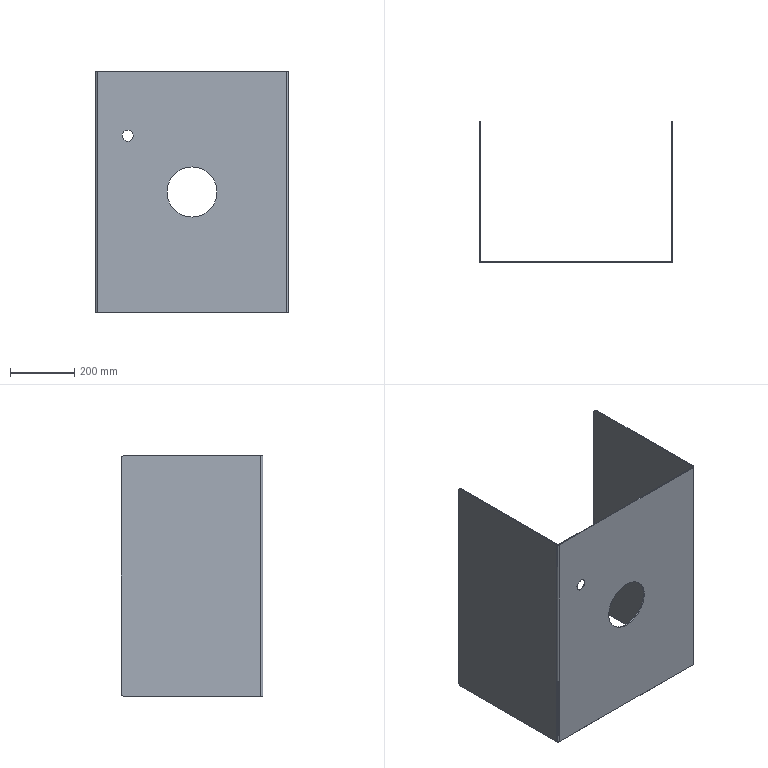Part | SolidWorks | features ICE 2, FlatPattern 1, SMBaseFlange 1, SheetMetal 1 | 1 solid | 30 faces | box 600 x 440 x 750 mm | volume 3247324 mm3 | plane 18 | cylinder 12 | commonest cylinder face diameters 20 x4 6 x2 12 x2 35 x2 156 x2
STEP:
#1=CARTESIAN_POINT('',(300.,0.,297.));
#2=VERTEX_POINT('',#1);
#3=CARTESIAN_POINT('',(300.,0.,453.));
#4=VERTEX_POINT('',#3);
#5=CARTESIAN_POINT('',(300.,0.,375.));
#6=DIRECTION('',(0.,1.,0.));
#7=DIRECTION('',(0.,0.,1.));
#8=AXIS2_PLACEMENT_3D('',#5,#6,#7);
#9=CIRCLE('',#8,78.);
#10=EDGE_CURVE('',#2,#4,#9,.T.);
#11=ORIENTED_EDGE('',*,*,#10,.F.);
#12=CARTESIAN_POINT('',(300.,3.,297.));
#13=VERTEX_POINT('',#12);
#14=CARTESIAN_POINT('',(300.,-7.,297.));
#15=DIRECTION('',(0.,1.,0.));
#16=VECTOR('',#15,1000.);
#17=LINE('',#14,#16);
#18=EDGE_CURVE('',#2,#13,#17,.T.);
#19=ORIENTED_EDGE('',*,*,#18,.T.);
#20=CARTESIAN_POINT('',(300.,3.,453.));
#21=VERTEX_POINT('',#20);
#22=CARTESIAN_POINT('',(300.,3.,375.));
#23=DIRECTION('',(0.,1.,0.));
#24=DIRECTION('',(0.,0.,1.));
#25=AXIS2_PLACEMENT_3D('',#22,#23,#24);
#26=CIRCLE('',#25,78.);
#27=EDGE_CURVE('',#13,#21,#26,.T.);
#28=ORIENTED_EDGE('',*,*,#27,.T.);
#29=CARTESIAN_POINT('',(300.,-7.,453.));
#30=DIRECTION('',(0.,1.,0.));
#31=VECTOR('',#30,1000.);
#32=LINE('',#29,#31);
#33=EDGE_CURVE('',#4,#21,#32,.T.);
#34=ORIENTED_EDGE('',*,*,#33,.F.);
#35=EDGE_LOOP('',(#11,#19,#28,#34));
#36=FACE_OUTER_BOUND('',#35,.T.);
#37=CARTESIAN_POINT('',(300.,-7.,375.));
#38=DIRECTION('',(0.,1.,0.));
#39=DIRECTION('',(0.,0.,1.));
#40=AXIS2_PLACEMENT_3D('',#37,#38,#39);
#41=CYLINDRICAL_SURFACE('',#40,78.);
#42=ADVANCED_FACE('',(#36),#41,.F.);
#43=CARTESIAN_POINT('',(100.,0.,532.5));
#44=VERTEX_POINT('',#43);
#45=CARTESIAN_POINT('',(100.,0.,567.5));
#46=VERTEX_POINT('',#45);
#47=CARTESIAN_POINT('',(100.,0.,550.));
#48=DIRECTION('',(0.,1.,0.));
#49=DIRECTION('',(0.,0.,1.));
#50=AXIS2_PLACEMENT_3D('',#47,#48,#49);
#51=CIRCLE('',#50,17.5);
#52=EDGE_CURVE('',#44,#46,#51,.T.);
#53=ORIENTED_EDGE('',*,*,#52,.F.);
#54=CARTESIAN_POINT('',(100.,3.,532.5));
#55=VERTEX_POINT('',#54);
#56=CARTESIAN_POINT('',(100.,-7.,532.5));
#57=DIRECTION('',(0.,1.,0.));
#58=VECTOR('',#57,1000.);
#59=LINE('',#56,#58);
#60=EDGE_CURVE('',#44,#55,#59,.T.);
#61=ORIENTED_EDGE('',*,*,#60,.T.);
#62=CARTESIAN_POINT('',(100.,3.,567.5));
#63=VERTEX_POINT('',#62);
#64=CARTESIAN_POINT('',(100.,3.,550.));
#65=DIRECTION('',(0.,1.,0.));
#66=DIRECTION('',(0.,0.,1.));
#67=AXIS2_PLACEMENT_3D('',#64,#65,#66);
#68=CIRCLE('',#67,17.5);
#69=EDGE_CURVE('',#55,#63,#68,.T.);
#70=ORIENTED_EDGE('',*,*,#69,.T.);
#71=CARTESIAN_POINT('',(100.,-7.,567.5));
#72=DIRECTION('',(0.,1.,0.));
#73=VECTOR('',#72,1000.);
#74=LINE('',#71,#73);
#75=EDGE_CURVE('',#46,#63,#74,.T.);
#76=ORIENTED_EDGE('',*,*,#75,.F.);
#77=EDGE_LOOP('',(#53,#61,#70,#76));
#78=FACE_OUTER_BOUND('',#77,.T.);
#79=CARTESIAN_POINT('',(100.,-7.,550.));
#80=DIRECTION('',(0.,1.,0.));
#81=DIRECTION('',(0.,0.,1.));
#82=AXIS2_PLACEMENT_3D('',#79,#80,#81);
#83=CYLINDRICAL_SURFACE('',#82,17.5);
#84=ADVANCED_FACE('',(#78),#83,.F.);
#85=CARTESIAN_POINT('',(600.,430.,0.));
#86=VERTEX_POINT('',#85);
#87=CARTESIAN_POINT('',(600.,440.,10.));
#88=VERTEX_POINT('',#87);
#89=CARTESIAN_POINT('',(600.,430.,10.));
#90=DIRECTION('',(1.,0.,0.));
#91=DIRECTION('',(0.,0.,1.));
#92=AXIS2_PLACEMENT_3D('',#89,#90,#91);
#93=CIRCLE('',#92,10.);
#94=EDGE_CURVE('',#86,#88,#93,.T.);
#95=ORIENTED_EDGE('',*,*,#94,.T.);
#96=CARTESIAN_POINT('',(600.,440.,740.));
#97=VERTEX_POINT('',#96);
#98=CARTESIAN_POINT('',(600.,440.,750.));
#99=DIRECTION('',(0.,0.,-1.));
#100=VECTOR('',#99,1000.);
#101=LINE('',#98,#100);
#102=EDGE_CURVE('',#97,#88,#101,.T.);
#103=ORIENTED_EDGE('',*,*,#102,.F.);
#104=CARTESIAN_POINT('',(600.,430.,750.));
#105=VERTEX_POINT('',#104);
#106=CARTESIAN_POINT('',(600.,430.,740.));
#107=DIRECTION('',(1.,0.,0.));
#108=DIRECTION('',(0.,0.,1.));
#109=AXIS2_PLACEMENT_3D('',#106,#107,#108);
#110=CIRCLE('',#109,10.);
#111=EDGE_CURVE('',#97,#105,#110,.T.);
#112=ORIENTED_EDGE('',*,*,#111,.T.);
#113=CARTESIAN_POINT('',(600.,6.,750.));
#114=VERTEX_POINT('',#113);
#115=CARTESIAN_POINT('',(600.,0.,750.));
#116=DIRECTION('',(0.,1.,0.));
#117=VECTOR('',#116,1000.);
#118=LINE('',#115,#117);
#119=EDGE_CURVE('',#114,#105,#118,.T.);
#120=ORIENTED_EDGE('',*,*,#119,.F.);
#121=CARTESIAN_POINT('',(600.,6.,0.));
#122=VERTEX_POINT('',#121);
#123=CARTESIAN_POINT('',(600.,6.,750.));
#124=DIRECTION('',(0.,0.,-1.));
#125=VECTOR('',#124,1000.);
#126=LINE('',#123,#125);
#127=EDGE_CURVE('',#114,#122,#126,.T.);
#128=ORIENTED_EDGE('',*,*,#127,.T.);
#129=CARTESIAN_POINT('',(600.,0.,0.));
#130=DIRECTION('',(0.,1.,0.));
#131=VECTOR('',#130,1000.);
#132=LINE('',#129,#131);
#133=EDGE_CURVE('',#122,#86,#132,.T.);
#134=ORIENTED_EDGE('',*,*,#133,.T.);
#135=EDGE_LOOP('',(#95,#103,#112,#120,#128,#134));
#136=FACE_OUTER_BOUND('',#135,.T.);
#137=CARTESIAN_POINT('',(600.,0.,750.));
#138=DIRECTION('',(-1.,0.,0.));
#139=DIRECTION('',(0.,0.,1.));
#140=AXIS2_PLACEMENT_3D('',#137,#138,#139);
#141=PLANE('',#140);
#142=ADVANCED_FACE('',(#136),#141,.F.);
#143=CARTESIAN_POINT('',(597.,440.,740.));
#144=VERTEX_POINT('',#143);
#145=CARTESIAN_POINT('',(597.,440.,10.));
#146=VERTEX_POINT('',#145);
#147=CARTESIAN_POINT('',(597.,440.,750.));
#148=DIRECTION('',(0.,0.,-1.));
#149=VECTOR('',#148,1000.);
#150=LINE('',#147,#149);
#151=EDGE_CURVE('',#144,#146,#150,.T.);
#152=ORIENTED_EDGE('',*,*,#151,.T.);
#153=CARTESIAN_POINT('',(597.,430.,0.));
#154=VERTEX_POINT('',#153);
#155=CARTESIAN_POINT('',(597.,430.,10.));
#156=DIRECTION('',(1.,0.,0.));
#157=DIRECTION('',(0.,0.,1.));
#158=AXIS2_PLACEMENT_3D('',#155,#156,#157);
#159=CIRCLE('',#158,10.);
#160=EDGE_CURVE('',#154,#146,#159,.T.);
#161=ORIENTED_EDGE('',*,*,#160,.F.);
#162=CARTESIAN_POINT('',(597.,6.,0.));
#163=VERTEX_POINT('',#162);
#164=CARTESIAN_POINT('',(597.,0.,0.));
#165=DIRECTION('',(0.,1.,0.));
#166=VECTOR('',#165,1000.);
#167=LINE('',#164,#166);
#168=EDGE_CURVE('',#163,#154,#167,.T.);
#169=ORIENTED_EDGE('',*,*,#168,.F.);
#170=CARTESIAN_POINT('',(597.,6.,750.));
#171=VERTEX_POINT('',#170);
#172=CARTESIAN_POINT('',(597.,6.,750.));
#173=DIRECTION('',(0.,0.,-1.));
#174=VECTOR('',#173,1000.);
#175=LINE('',#172,#174);
#176=EDGE_CURVE('',#171,#163,#175,.T.);
#177=ORIENTED_EDGE('',*,*,#176,.F.);
#178=CARTESIAN_POINT('',(597.,430.,750.));
#179=VERTEX_POINT('',#178);
#180=CARTESIAN_POINT('',(597.,0.,750.));
#181=DIRECTION('',(0.,1.,0.));
#182=VECTOR('',#181,1000.);
#183=LINE('',#180,#182);
#184=EDGE_CURVE('',#171,#179,#183,.T.);
#185=ORIENTED_EDGE('',*,*,#184,.T.);
#186=CARTESIAN_POINT('',(597.,430.,740.));
#187=DIRECTION('',(1.,0.,0.));
#188=DIRECTION('',(0.,0.,1.));
#189=AXIS2_PLACEMENT_3D('',#186,#187,#188);
#190=CIRCLE('',#189,10.);
#191=EDGE_CURVE('',#144,#179,#190,.T.);
#192=ORIENTED_EDGE('',*,*,#191,.F.);
#193=EDGE_LOOP('',(#152,#161,#169,#177,#185,#192));
#194=FACE_OUTER_BOUND('',#193,.T.);
#195=CARTESIAN_POINT('',(597.,0.,750.));
#196=DIRECTION('',(-1.,0.,0.));
#197=DIRECTION('',(0.,0.,1.));
#198=AXIS2_PLACEMENT_3D('',#195,#196,#197);
#199=PLANE('',#198);
#200=ADVANCED_FACE('',(#194),#199,.T.);
#201=ORIENTED_EDGE('',*,*,#102,.T.);
#202=CARTESIAN_POINT('',(597.,440.,10.));
#203=DIRECTION('',(1.,0.,0.));
#204=VECTOR('',#203,1000.);
#205=LINE('',#202,#204);
#206=EDGE_CURVE('',#146,#88,#205,.T.);
#207=ORIENTED_EDGE('',*,*,#206,.F.);
#208=ORIENTED_EDGE('',*,*,#151,.F.);
#209=CARTESIAN_POINT('',(597.,440.,740.));
#210=DIRECTION('',(1.,0.,0.));
#211=VECTOR('',#210,1000.);
#212=LINE('',#209,#211);
#213=EDGE_CURVE('',#144,#97,#212,.T.);
#214=ORIENTED_EDGE('',*,*,#213,.T.);
#215=EDGE_LOOP('',(#201,#207,#208,#214));
#216=FACE_OUTER_BOUND('',#215,.T.);
#217=CARTESIAN_POINT('',(597.,440.,750.));
#218=DIRECTION('',(0.,1.,0.));
#219=DIRECTION('',(0.,0.,1.));
#220=AXIS2_PLACEMENT_3D('',#217,#218,#219);
#221=PLANE('',#220);
#222=ADVANCED_FACE('',(#216),#221,.T.);
#223=CARTESIAN_POINT('',(3.,430.,0.));
#224=VERTEX_POINT('',#223);
#225=CARTESIAN_POINT('',(3.,6.,0.));
#226=VERTEX_POINT('',#225);
#227=CARTESIAN_POINT('',(3.,0.,0.));
#228=DIRECTION('',(0.,-1.,0.));
#229=VECTOR('',#228,1000.);
#230=LINE('',#227,#229);
#231=EDGE_CURVE('',#224,#226,#230,.T.);
#232=ORIENTED_EDGE('',*,*,#231,.F.);
#233=CARTESIAN_POINT('',(3.,440.,10.));
#234=VERTEX_POINT('',#233);
#235=CARTESIAN_POINT('',(3.,430.,10.));
#236=DIRECTION('',(-1.,0.,0.));
#237=DIRECTION('',(0.,0.,-1.));
#238=AXIS2_PLACEMENT_3D('',#235,#236,#237);
#239=CIRCLE('',#238,10.);
#240=EDGE_CURVE('',#234,#224,#239,.T.);
#241=ORIENTED_EDGE('',*,*,#240,.F.);
#242=CARTESIAN_POINT('',(3.,440.,740.));
#243=VERTEX_POINT('',#242);
#244=CARTESIAN_POINT('',(3.,440.,750.));
#245=DIRECTION('',(0.,0.,-1.));
#246=VECTOR('',#245,1000.);
#247=LINE('',#244,#246);
#248=EDGE_CURVE('',#243,#234,#247,.T.);
#249=ORIENTED_EDGE('',*,*,#248,.F.);
#250=CARTESIAN_POINT('',(3.,430.,750.));
#251=VERTEX_POINT('',#250);
#252=CARTESIAN_POINT('',(3.,430.,740.));
#253=DIRECTION('',(-1.,0.,0.));
#254=DIRECTION('',(0.,0.,-1.));
#255=AXIS2_PLACEMENT_3D('',#252,#253,#254);
#256=CIRCLE('',#255,10.);
#257=EDGE_CURVE('',#251,#243,#256,.T.);
#258=ORIENTED_EDGE('',*,*,#257,.F.);
#259=CARTESIAN_POINT('',(3.,6.,750.));
#260=VERTEX_POINT('',#259);
#261=CARTESIAN_POINT('',(3.,0.,750.));
#262=DIRECTION('',(0.,-1.,0.));
#263=VECTOR('',#262,1000.);
#264=LINE('',#261,#263);
#265=EDGE_CURVE('',#251,#260,#264,.T.);
#266=ORIENTED_EDGE('',*,*,#265,.T.);
#267=CARTESIAN_POINT('',(3.,6.,750.));
#268=DIRECTION('',(0.,0.,-1.));
#269=VECTOR('',#268,1000.);
#270=LINE('',#267,#269);
#271=EDGE_CURVE('',#260,#226,#270,.T.);
#272=ORIENTED_EDGE('',*,*,#271,.T.);
#273=EDGE_LOOP('',(#232,#241,#249,#258,#266,#272));
#274=FACE_OUTER_BOUND('',#273,.T.);
#275=CARTESIAN_POINT('',(3.,0.,750.));
#276=DIRECTION('',(1.,0.,0.));
#277=DIRECTION('',(0.,0.,-1.));
#278=AXIS2_PLACEMENT_3D('',#275,#276,#277);
#279=PLANE('',#278);
#280=ADVANCED_FACE('',(#274),#279,.T.);
#281=CARTESIAN_POINT('',(0.,440.,10.));
#282=VERTEX_POINT('',#281);
#283=CARTESIAN_POINT('',(0.,430.,0.));
#284=VERTEX_POINT('',#283);
#285=CARTESIAN_POINT('',(0.,430.,10.));
#286=DIRECTION('',(-1.,0.,0.));
#287=DIRECTION('',(0.,0.,-1.));
#288=AXIS2_PLACEMENT_3D('',#285,#286,#287);
#289=CIRCLE('',#288,10.);
#290=EDGE_CURVE('',#282,#284,#289,.T.);
#291=ORIENTED_EDGE('',*,*,#290,.T.);
#292=CARTESIAN_POINT('',(0.,6.,0.));
#293=VERTEX_POINT('',#292);
#294=CARTESIAN_POINT('',(0.,0.,0.));
#295=DIRECTION('',(0.,-1.,0.));
#296=VECTOR('',#295,1000.);
#297=LINE('',#294,#296);
#298=EDGE_CURVE('',#284,#293,#297,.T.);
#299=ORIENTED_EDGE('',*,*,#298,.T.);
#300=CARTESIAN_POINT('',(0.,6.,750.));
#301=VERTEX_POINT('',#300);
#302=CARTESIAN_POINT('',(0.,6.,750.));
#303=DIRECTION('',(0.,0.,-1.));
#304=VECTOR('',#303,1000.);
#305=LINE('',#302,#304);
#306=EDGE_CURVE('',#301,#293,#305,.T.);
#307=ORIENTED_EDGE('',*,*,#306,.F.);
#308=CARTESIAN_POINT('',(0.,430.,750.));
#309=VERTEX_POINT('',#308);
#310=CARTESIAN_POINT('',(0.,0.,750.));
#311=DIRECTION('',(0.,-1.,0.));
#312=VECTOR('',#311,1000.);
#313=LINE('',#310,#312);
#314=EDGE_CURVE('',#309,#301,#313,.T.);
#315=ORIENTED_EDGE('',*,*,#314,.F.);
#316=CARTESIAN_POINT('',(0.,440.,740.));
#317=VERTEX_POINT('',#316);
#318=CARTESIAN_POINT('',(0.,430.,740.));
#319=DIRECTION('',(-1.,0.,0.));
#320=DIRECTION('',(0.,0.,-1.));
#321=AXIS2_PLACEMENT_3D('',#318,#319,#320);
#322=CIRCLE('',#321,10.);
#323=EDGE_CURVE('',#309,#317,#322,.T.);
#324=ORIENTED_EDGE('',*,*,#323,.T.);
#325=CARTESIAN_POINT('',(0.,440.,750.));
#326=DIRECTION('',(0.,0.,-1.));
#327=VECTOR('',#326,1000.);
#328=LINE('',#325,#327);
#329=EDGE_CURVE('',#317,#282,#328,.T.);
#330=ORIENTED_EDGE('',*,*,#329,.T.);
#331=EDGE_LOOP('',(#291,#299,#307,#315,#324,#330));
#332=FACE_OUTER_BOUND('',#331,.T.);
#333=CARTESIAN_POINT('',(0.,0.,750.));
#334=DIRECTION('',(1.,0.,0.));
#335=DIRECTION('',(0.,0.,-1.));
#336=AXIS2_PLACEMENT_3D('',#333,#334,#335);
#337=PLANE('',#336);
#338=ADVANCED_FACE('',(#332),#337,.F.);
#339=ORIENTED_EDGE('',*,*,#119,.T.);
#340=CARTESIAN_POINT('',(597.,430.,750.));
#341=DIRECTION('',(1.,0.,0.));
#342=VECTOR('',#341,1000.);
#343=LINE('',#340,#342);
#344=EDGE_CURVE('',#179,#105,#343,.T.);
#345=ORIENTED_EDGE('',*,*,#344,.F.);
#346=ORIENTED_EDGE('',*,*,#184,.F.);
#347=CARTESIAN_POINT('',(597.,6.,750.));
#348=DIRECTION('',(1.,0.,0.));
#349=VECTOR('',#348,1000.);
#350=LINE('',#347,#349);
#351=EDGE_CURVE('',#171,#114,#350,.T.);
#352=ORIENTED_EDGE('',*,*,#351,.T.);
#353=EDGE_LOOP('',(#339,#345,#346,#352));
#354=FACE_OUTER_BOUND('',#353,.T.);
#355=CARTESIAN_POINT('',(594.,6.,750.));
#356=DIRECTION('',(0.,0.,1.));
#357=DIRECTION('',(1.,0.,0.));
#358=AXIS2_PLACEMENT_3D('',#355,#356,#357);
#359=PLANE('',#358);
#360=ADVANCED_FACE('',(#354),#359,.T.);
#361=CARTESIAN_POINT('',(3.,440.,10.));
#362=DIRECTION('',(-1.,0.,0.));
#363=VECTOR('',#362,1000.);
#364=LINE('',#361,#363);
#365=EDGE_CURVE('',#234,#282,#364,.T.);
#366=ORIENTED_EDGE('',*,*,#365,.T.);
#367=ORIENTED_EDGE('',*,*,#329,.F.);
#368=CARTESIAN_POINT('',(3.,440.,740.));
#369=DIRECTION('',(-1.,0.,0.));
#370=VECTOR('',#369,1000.);
#371=LINE('',#368,#370);
#372=EDGE_CURVE('',#243,#317,#371,.T.);
#373=ORIENTED_EDGE('',*,*,#372,.F.);
#374=ORIENTED_EDGE('',*,*,#248,.T.);
#375=EDGE_LOOP('',(#366,#367,#373,#374));
#376=FACE_OUTER_BOUND('',#375,.T.);
#377=CARTESIAN_POINT('',(0.,440.,750.));
#378=DIRECTION('',(0.,1.,0.));
#379=DIRECTION('',(0.,0.,1.));
#380=AXIS2_PLACEMENT_3D('',#377,#378,#379);
#381=PLANE('',#380);
#382=ADVANCED_FACE('',(#376),#381,.T.);
#383=CARTESIAN_POINT('',(0.,6.,750.));
#384=DIRECTION('',(1.,0.,0.));
#385=VECTOR('',#384,1000.);
#386=LINE('',#383,#385);
#387=EDGE_CURVE('',#301,#260,#386,.T.);
#388=ORIENTED_EDGE('',*,*,#387,.F.);
#389=CARTESIAN_POINT('',(6.,0.,750.));
#390=VERTEX_POINT('',#389);
#391=CARTESIAN_POINT('',(6.,6.,750.));
#392=DIRECTION('',(0.,0.,1.));
#393=DIRECTION('',(-1.,0.,0.));
#394=AXIS2_PLACEMENT_3D('',#391,#392,#393);
#395=CIRCLE('',#394,6.);
#396=EDGE_CURVE('',#301,#390,#395,.T.);
#397=ORIENTED_EDGE('',*,*,#396,.T.);
#398=CARTESIAN_POINT('',(6.,3.,750.));
#399=VERTEX_POINT('',#398);
#400=CARTESIAN_POINT('',(6.,3.,750.));
#401=DIRECTION('',(0.,-1.,0.));
#402=VECTOR('',#401,1000.);
#403=LINE('',#400,#402);
#404=EDGE_CURVE('',#399,#390,#403,.T.);
#405=ORIENTED_EDGE('',*,*,#404,.F.);
#406=CARTESIAN_POINT('',(6.,6.,750.));
#407=DIRECTION('',(0.,0.,1.));
#408=DIRECTION('',(1.,0.,0.));
#409=AXIS2_PLACEMENT_3D('',#406,#407,#408);
#410=CIRCLE('',#409,3.);
#411=EDGE_CURVE('',#260,#399,#410,.T.);
#412=ORIENTED_EDGE('',*,*,#411,.F.);
#413=EDGE_LOOP('',(#388,#397,#405,#412));
#414=FACE_OUTER_BOUND('',#413,.T.);
#415=CARTESIAN_POINT('',(0.,6.,750.));
#416=DIRECTION('',(0.,0.,1.));
#417=DIRECTION('',(1.,0.,0.));
#418=AXIS2_PLACEMENT_3D('',#415,#416,#417);
#419=PLANE('',#418);
#420=ADVANCED_FACE('',(#414),#419,.T.);
#421=CARTESIAN_POINT('',(3.,430.,750.));
#422=DIRECTION('',(-1.,0.,0.));
#423=VECTOR('',#422,1000.);
#424=LINE('',#421,#423);
#425=EDGE_CURVE('',#251,#309,#424,.T.);
#426=ORIENTED_EDGE('',*,*,#425,.T.);
#427=ORIENTED_EDGE('',*,*,#314,.T.);
#428=ORIENTED_EDGE('',*,*,#387,.T.);
#429=ORIENTED_EDGE('',*,*,#265,.F.);
#430=EDGE_LOOP('',(#426,#427,#428,#429));
#431=FACE_OUTER_BOUND('',#430,.T.);
#432=CARTESIAN_POINT('',(6.,3.,750.));
#433=DIRECTION('',(0.,0.,1.));
#434=DIRECTION('',(1.,0.,0.));
#435=AXIS2_PLACEMENT_3D('',#432,#433,#434);
#436=PLANE('',#435);
#437=ADVANCED_FACE('',(#431),#436,.T.);
#438=CARTESIAN_POINT('',(6.,0.,0.));
#439=VERTEX_POINT('',#438);
#440=CARTESIAN_POINT('',(6.,3.,0.));
#441=VERTEX_POINT('',#440);
#442=CARTESIAN_POINT('',(6.,0.,0.));
#443=DIRECTION('',(0.,1.,0.));
#444=VECTOR('',#443,1000.);
#445=LINE('',#442,#444);
#446=EDGE_CURVE('',#439,#441,#445,.T.);
#447=ORIENTED_EDGE('',*,*,#446,.F.);
#448=CARTESIAN_POINT('',(6.,6.,0.));
#449=DIRECTION('',(0.,0.,1.));
#450=DIRECTION('',(-1.,0.,0.));
#451=AXIS2_PLACEMENT_3D('',#448,#449,#450);
#452=CIRCLE('',#451,6.);
#453=EDGE_CURVE('',#293,#439,#452,.T.);
#454=ORIENTED_EDGE('',*,*,#453,.F.);
#455=CARTESIAN_POINT('',(3.,6.,0.));
#456=DIRECTION('',(-1.,0.,0.));
#457=VECTOR('',#456,1000.);
#458=LINE('',#455,#457);
#459=EDGE_CURVE('',#226,#293,#458,.T.);
#460=ORIENTED_EDGE('',*,*,#459,.F.);
#461=CARTESIAN_POINT('',(6.,6.,0.));
#462=DIRECTION('',(0.,0.,1.));
#463=DIRECTION('',(1.,0.,0.));
#464=AXIS2_PLACEMENT_3D('',#461,#462,#463);
#465=CIRCLE('',#464,3.);
#466=EDGE_CURVE('',#226,#441,#465,.T.);
#467=ORIENTED_EDGE('',*,*,#466,.T.);
#468=EDGE_LOOP('',(#447,#454,#460,#467));
#469=FACE_OUTER_BOUND('',#468,.T.);
#470=CARTESIAN_POINT('',(6.,0.,0.));
#471=DIRECTION('',(0.,0.,-1.));
#472=DIRECTION('',(-1.,0.,0.));
#473=AXIS2_PLACEMENT_3D('',#470,#471,#472);
#474=PLANE('',#473);
#475=ADVANCED_FACE('',(#469),#474,.T.);
#476=CARTESIAN_POINT('',(594.,0.,0.));
#477=VERTEX_POINT('',#476);
#478=CARTESIAN_POINT('',(0.,0.,0.));
#479=DIRECTION('',(1.,0.,0.));
#480=VECTOR('',#479,1000.);
#481=LINE('',#478,#480);
#482=EDGE_CURVE('',#439,#477,#481,.T.);
#483=ORIENTED_EDGE('',*,*,#482,.F.);
#484=ORIENTED_EDGE('',*,*,#446,.T.);
#485=CARTESIAN_POINT('',(594.,3.,0.));
#486=VERTEX_POINT('',#485);
#487=CARTESIAN_POINT('',(0.,3.,0.));
#488=DIRECTION('',(1.,0.,0.));
#489=VECTOR('',#488,1000.);
#490=LINE('',#487,#489);
#491=EDGE_CURVE('',#441,#486,#490,.T.);
#492=ORIENTED_EDGE('',*,*,#491,.T.);
#493=CARTESIAN_POINT('',(594.,3.,0.));
#494=DIRECTION('',(0.,-1.,0.));
#495=VECTOR('',#494,1000.);
#496=LINE('',#493,#495);
#497=EDGE_CURVE('',#486,#477,#496,.T.);
#498=ORIENTED_EDGE('',*,*,#497,.T.);
#499=EDGE_LOOP('',(#483,#484,#492,#498));
#500=FACE_OUTER_BOUND('',#499,.T.);
#501=CARTESIAN_POINT('',(3.,6.,0.));
#502=DIRECTION('',(0.,0.,-1.));
#503=DIRECTION('',(-1.,0.,0.));
#504=AXIS2_PLACEMENT_3D('',#501,#502,#503);
#505=PLANE('',#504);
#506=ADVANCED_FACE('',(#500),#505,.T.);
#507=CARTESIAN_POINT('',(594.,0.,750.));
#508=VERTEX_POINT('',#507);
#509=CARTESIAN_POINT('',(594.,3.,750.));
#510=VERTEX_POINT('',#509);
#511=CARTESIAN_POINT('',(594.,0.,750.));
#512=DIRECTION('',(0.,1.,0.));
#513=VECTOR('',#512,1000.);
#514=LINE('',#511,#513);
#515=EDGE_CURVE('',#508,#510,#514,.T.);
#516=ORIENTED_EDGE('',*,*,#515,.F.);
#517=CARTESIAN_POINT('',(594.,6.,750.));
#518=DIRECTION('',(0.,0.,1.));
#519=DIRECTION('',(-1.,0.,0.));
#520=AXIS2_PLACEMENT_3D('',#517,#518,#519);
#521=CIRCLE('',#520,6.);
#522=EDGE_CURVE('',#508,#114,#521,.T.);
#523=ORIENTED_EDGE('',*,*,#522,.T.);
#524=ORIENTED_EDGE('',*,*,#351,.F.);
#525=CARTESIAN_POINT('',(594.,6.,750.));
#526=DIRECTION('',(0.,0.,1.));
#527=DIRECTION('',(1.,0.,0.));
#528=AXIS2_PLACEMENT_3D('',#525,#526,#527);
#529=CIRCLE('',#528,3.);
#530=EDGE_CURVE('',#510,#171,#529,.T.);
#531=ORIENTED_EDGE('',*,*,#530,.F.);
#532=EDGE_LOOP('',(#516,#523,#524,#531));
#533=FACE_OUTER_BOUND('',#532,.T.);
#534=CARTESIAN_POINT('',(594.,0.,750.));
#535=DIRECTION('',(0.,0.,1.));
#536=DIRECTION('',(1.,0.,0.));
#537=AXIS2_PLACEMENT_3D('',#534,#535,#536);
#538=PLANE('',#537);
#539=ADVANCED_FACE('',(#533),#538,.T.);
#540=CARTESIAN_POINT('',(0.,0.,750.));
#541=DIRECTION('',(1.,0.,0.));
#542=VECTOR('',#541,1000.);
#543=LINE('',#540,#542);
#544=EDGE_CURVE('',#390,#508,#543,.T.);
#545=ORIENTED_EDGE('',*,*,#544,.T.);
#546=ORIENTED_EDGE('',*,*,#515,.T.);
#547=CARTESIAN_POINT('',(0.,3.,750.));
#548=DIRECTION('',(1.,0.,0.));
#549=VECTOR('',#548,1000.);
#550=LINE('',#547,#549);
#551=EDGE_CURVE('',#399,#510,#550,.T.);
#552=ORIENTED_EDGE('',*,*,#551,.F.);
#553=ORIENTED_EDGE('',*,*,#404,.T.);
#554=EDGE_LOOP('',(#545,#546,#552,#553));
#555=FACE_OUTER_BOUND('',#554,.T.);
#556=CARTESIAN_POINT('',(597.,6.,750.));
#557=DIRECTION('',(0.,0.,1.));
#558=DIRECTION('',(1.,0.,0.));
#559=AXIS2_PLACEMENT_3D('',#556,#557,#558);
#560=PLANE('',#559);
#561=ADVANCED_FACE('',(#555),#560,.T.);
#562=CARTESIAN_POINT('',(600.,6.,0.));
#563=DIRECTION('',(-1.,0.,0.));
#564=VECTOR('',#563,1000.);
#565=LINE('',#562,#564);
#566=EDGE_CURVE('',#122,#163,#565,.T.);
#567=ORIENTED_EDGE('',*,*,#566,.F.);
#568=CARTESIAN_POINT('',(594.,6.,0.));
#569=DIRECTION('',(0.,0.,1.));
#570=DIRECTION('',(-1.,0.,0.));
#571=AXIS2_PLACEMENT_3D('',#568,#569,#570);
#572=CIRCLE('',#571,6.);
#573=EDGE_CURVE('',#477,#122,#572,.T.);
#574=ORIENTED_EDGE('',*,*,#573,.F.);
#575=ORIENTED_EDGE('',*,*,#497,.F.);
#576=CARTESIAN_POINT('',(594.,6.,0.));
#577=DIRECTION('',(0.,0.,1.));
#578=DIRECTION('',(1.,0.,0.));
#579=AXIS2_PLACEMENT_3D('',#576,#577,#578);
#580=CIRCLE('',#579,3.);
#581=EDGE_CURVE('',#486,#163,#580,.T.);
#582=ORIENTED_EDGE('',*,*,#581,.T.);
#583=EDGE_LOOP('',(#567,#574,#575,#582));
#584=FACE_OUTER_BOUND('',#583,.T.);
#585=CARTESIAN_POINT('',(600.,6.,0.));
#586=DIRECTION('',(0.,0.,-1.));
#587=DIRECTION('',(-1.,0.,0.));
#588=AXIS2_PLACEMENT_3D('',#585,#586,#587);
#589=PLANE('',#588);
#590=ADVANCED_FACE('',(#584),#589,.T.);
#591=CARTESIAN_POINT('',(597.,430.,0.));
#592=DIRECTION('',(1.,0.,0.));
#593=VECTOR('',#592,1000.);
#594=LINE('',#591,#593);
#595=EDGE_CURVE('',#154,#86,#594,.T.);
#596=ORIENTED_EDGE('',*,*,#595,.T.);
#597=ORIENTED_EDGE('',*,*,#133,.F.);
#598=ORIENTED_EDGE('',*,*,#566,.T.);
#599=ORIENTED_EDGE('',*,*,#168,.T.);
#600=EDGE_LOOP('',(#596,#597,#598,#599));
#601=FACE_OUTER_BOUND('',#600,.T.);
#602=CARTESIAN_POINT('',(594.,3.,0.));
#603=DIRECTION('',(0.,0.,-1.));
#604=DIRECTION('',(-1.,0.,0.));
#605=AXIS2_PLACEMENT_3D('',#602,#603,#604);
#606=PLANE('',#605);
#607=ADVANCED_FACE('',(#601),#606,.T.);
#608=ORIENTED_EDGE('',*,*,#581,.F.);
#609=CARTESIAN_POINT('',(594.,3.,750.));
#610=DIRECTION('',(0.,0.,-1.));
#611=VECTOR('',#610,1000.);
#612=LINE('',#609,#611);
#613=EDGE_CURVE('',#510,#486,#612,.T.);
#614=ORIENTED_EDGE('',*,*,#613,.F.);
#615=ORIENTED_EDGE('',*,*,#530,.T.);
#616=ORIENTED_EDGE('',*,*,#176,.T.);
#617=EDGE_LOOP('',(#608,#614,#615,#616));
#618=FACE_OUTER_BOUND('',#617,.T.);
#619=CARTESIAN_POINT('',(594.,6.,750.));
#620=DIRECTION('',(0.,0.,-1.));
#621=DIRECTION('',(-1.,0.,0.));
#622=AXIS2_PLACEMENT_3D('',#619,#620,#621);
#623=CYLINDRICAL_SURFACE('',#622,3.);
#624=ADVANCED_FACE('',(#618),#623,.F.);
#625=CARTESIAN_POINT('',(300.,3.,375.));
#626=DIRECTION('',(0.,1.,0.));
#627=DIRECTION('',(0.,0.,1.));
#628=AXIS2_PLACEMENT_3D('',#625,#626,#627);
#629=CIRCLE('',#628,78.);
#630=EDGE_CURVE('',#21,#13,#629,.T.);
#631=ORIENTED_EDGE('',*,*,#630,.F.);
#632=ORIENTED_EDGE('',*,*,#27,.F.);
#633=EDGE_LOOP('',(#631,#632));
#634=FACE_BOUND('',#633,.T.);
#635=CARTESIAN_POINT('',(100.,3.,550.));
#636=DIRECTION('',(0.,1.,0.));
#637=DIRECTION('',(0.,0.,1.));
#638=AXIS2_PLACEMENT_3D('',#635,#636,#637);
#639=CIRCLE('',#638,17.5);
#640=EDGE_CURVE('',#63,#55,#639,.T.);
#641=ORIENTED_EDGE('',*,*,#640,.F.);
#642=ORIENTED_EDGE('',*,*,#69,.F.);
#643=EDGE_LOOP('',(#641,#642));
#644=FACE_BOUND('',#643,.T.);
#645=ORIENTED_EDGE('',*,*,#491,.F.);
#646=CARTESIAN_POINT('',(6.,3.,750.));
#647=DIRECTION('',(0.,0.,-1.));
#648=VECTOR('',#647,1000.);
#649=LINE('',#646,#648);
#650=EDGE_CURVE('',#399,#441,#649,.T.);
#651=ORIENTED_EDGE('',*,*,#650,.F.);
#652=ORIENTED_EDGE('',*,*,#551,.T.);
#653=ORIENTED_EDGE('',*,*,#613,.T.);
#654=EDGE_LOOP('',(#645,#651,#652,#653));
#655=FACE_OUTER_BOUND('',#654,.T.);
#656=CARTESIAN_POINT('',(0.,3.,750.));
#657=DIRECTION('',(0.,1.,0.));
#658=DIRECTION('',(0.,0.,1.));
#659=AXIS2_PLACEMENT_3D('',#656,#657,#658);
#660=PLANE('',#659);
#661=ADVANCED_FACE('',(#634,#644,#655),#660,.T.);
#662=ORIENTED_EDGE('',*,*,#466,.F.);
#663=ORIENTED_EDGE('',*,*,#271,.F.);
#664=ORIENTED_EDGE('',*,*,#411,.T.);
#665=ORIENTED_EDGE('',*,*,#650,.T.);
#666=EDGE_LOOP('',(#662,#663,#664,#665));
#667=FACE_OUTER_BOUND('',#666,.T.);
#668=CARTESIAN_POINT('',(6.,6.,750.));
#669=DIRECTION('',(0.,0.,-1.));
#670=DIRECTION('',(-1.,0.,0.));
#671=AXIS2_PLACEMENT_3D('',#668,#669,#670);
#672=CYLINDRICAL_SURFACE('',#671,3.);
#673=ADVANCED_FACE('',(#667),#672,.F.);
#674=ORIENTED_EDGE('',*,*,#453,.T.);
#675=CARTESIAN_POINT('',(6.,0.,750.));
#676=DIRECTION('',(0.,0.,-1.));
#677=VECTOR('',#676,1000.);
#678=LINE('',#675,#677);
#679=EDGE_CURVE('',#390,#439,#678,.T.);
#680=ORIENTED_EDGE('',*,*,#679,.F.);
#681=ORIENTED_EDGE('',*,*,#396,.F.);
#682=ORIENTED_EDGE('',*,*,#306,.T.);
#683=EDGE_LOOP('',(#674,#680,#681,#682));
#684=FACE_OUTER_BOUND('',#683,.T.);
#685=CARTESIAN_POINT('',(6.,6.,750.));
#686=DIRECTION('',(0.,0.,-1.));
#687=DIRECTION('',(-1.,0.,0.));
#688=AXIS2_PLACEMENT_3D('',#685,#686,#687);
#689=CYLINDRICAL_SURFACE('',#688,6.);
#690=ADVANCED_FACE('',(#684),#689,.T.);
#691=CARTESIAN_POINT('',(300.,0.,375.));
#692=DIRECTION('',(0.,1.,0.));
#693=DIRECTION('',(0.,0.,1.));
#694=AXIS2_PLACEMENT_3D('',#691,#692,#693);
#695=CIRCLE('',#694,78.);
#696=EDGE_CURVE('',#4,#2,#695,.T.);
#697=ORIENTED_EDGE('',*,*,#696,.T.);
#698=ORIENTED_EDGE('',*,*,#10,.T.);
#699=EDGE_LOOP('',(#697,#698));
#700=FACE_BOUND('',#699,.T.);
#701=CARTESIAN_POINT('',(100.,0.,550.));
#702=DIRECTION('',(0.,1.,0.));
#703=DIRECTION('',(0.,0.,1.));
#704=AXIS2_PLACEMENT_3D('',#701,#702,#703);
#705=CIRCLE('',#704,17.5);
#706=EDGE_CURVE('',#46,#44,#705,.T.);
#707=ORIENTED_EDGE('',*,*,#706,.T.);
#708=ORIENTED_EDGE('',*,*,#52,.T.);
#709=EDGE_LOOP('',(#707,#708));
#710=FACE_BOUND('',#709,.T.);
#711=ORIENTED_EDGE('',*,*,#482,.T.);
#712=CARTESIAN_POINT('',(594.,0.,750.));
#713=DIRECTION('',(0.,0.,-1.));
#714=VECTOR('',#713,1000.);
#715=LINE('',#712,#714);
#716=EDGE_CURVE('',#508,#477,#715,.T.);
#717=ORIENTED_EDGE('',*,*,#716,.F.);
#718=ORIENTED_EDGE('',*,*,#544,.F.);
#719=ORIENTED_EDGE('',*,*,#679,.T.);
#720=EDGE_LOOP('',(#711,#717,#718,#719));
#721=FACE_OUTER_BOUND('',#720,.T.);
#722=CARTESIAN_POINT('',(0.,0.,750.));
#723=DIRECTION('',(0.,1.,0.));
#724=DIRECTION('',(0.,0.,1.));
#725=AXIS2_PLACEMENT_3D('',#722,#723,#724);
#726=PLANE('',#725);
#727=ADVANCED_FACE('',(#700,#710,#721),#726,.F.);
#728=ORIENTED_EDGE('',*,*,#573,.T.);
#729=ORIENTED_EDGE('',*,*,#127,.F.);
#730=ORIENTED_EDGE('',*,*,#522,.F.);
#731=ORIENTED_EDGE('',*,*,#716,.T.);
#732=EDGE_LOOP('',(#728,#729,#730,#731));
#733=FACE_OUTER_BOUND('',#732,.T.);
#734=CARTESIAN_POINT('',(594.,6.,750.));
#735=DIRECTION('',(0.,0.,-1.));
#736=DIRECTION('',(-1.,0.,0.));
#737=AXIS2_PLACEMENT_3D('',#734,#735,#736);
#738=CYLINDRICAL_SURFACE('',#737,6.);
#739=ADVANCED_FACE('',(#733),#738,.T.);
#740=ORIENTED_EDGE('',*,*,#298,.F.);
#741=CARTESIAN_POINT('',(3.,430.,0.));
#742=DIRECTION('',(-1.,0.,0.));
#743=VECTOR('',#742,1000.);
#744=LINE('',#741,#743);
#745=EDGE_CURVE('',#224,#284,#744,.T.);
#746=ORIENTED_EDGE('',*,*,#745,.F.);
#747=ORIENTED_EDGE('',*,*,#231,.T.);
#748=ORIENTED_EDGE('',*,*,#459,.T.);
#749=EDGE_LOOP('',(#740,#746,#747,#748));
#750=FACE_OUTER_BOUND('',#749,.T.);
#751=CARTESIAN_POINT('',(594.,6.,0.));
#752=DIRECTION('',(0.,0.,1.));
#753=DIRECTION('',(1.,0.,0.));
#754=AXIS2_PLACEMENT_3D('',#751,#752,#753);
#755=PLANE('',#754);
#756=ADVANCED_FACE('',(#750),#755,.F.);
#757=ORIENTED_EDGE('',*,*,#60,.F.);
#758=ORIENTED_EDGE('',*,*,#706,.F.);
#759=ORIENTED_EDGE('',*,*,#75,.T.);
#760=ORIENTED_EDGE('',*,*,#640,.T.);
#761=EDGE_LOOP('',(#757,#758,#759,#760));
#762=FACE_OUTER_BOUND('',#761,.T.);
#763=CARTESIAN_POINT('',(100.,-7.,550.));
#764=DIRECTION('',(0.,1.,0.));
#765=DIRECTION('',(0.,0.,1.));
#766=AXIS2_PLACEMENT_3D('',#763,#764,#765);
#767=CYLINDRICAL_SURFACE('',#766,17.5);
#768=ADVANCED_FACE('',(#762),#767,.F.);
#769=ORIENTED_EDGE('',*,*,#18,.F.);
#770=ORIENTED_EDGE('',*,*,#696,.F.);
#771=ORIENTED_EDGE('',*,*,#33,.T.);
#772=ORIENTED_EDGE('',*,*,#630,.T.);
#773=EDGE_LOOP('',(#769,#770,#771,#772));
#774=FACE_OUTER_BOUND('',#773,.T.);
#775=CARTESIAN_POINT('',(300.,-7.,375.));
#776=DIRECTION('',(0.,1.,0.));
#777=DIRECTION('',(0.,0.,1.));
#778=AXIS2_PLACEMENT_3D('',#775,#776,#777);
#779=CYLINDRICAL_SURFACE('',#778,78.);
#780=ADVANCED_FACE('',(#774),#779,.F.);
#781=ORIENTED_EDGE('',*,*,#257,.T.);
#782=ORIENTED_EDGE('',*,*,#372,.T.);
#783=ORIENTED_EDGE('',*,*,#323,.F.);
#784=ORIENTED_EDGE('',*,*,#425,.F.);
#785=EDGE_LOOP('',(#781,#782,#783,#784));
#786=FACE_OUTER_BOUND('',#785,.T.);
#787=CARTESIAN_POINT('',(3.,430.,740.));
#788=DIRECTION('',(1.,0.,0.));
#789=DIRECTION('',(0.,0.,-1.));
#790=AXIS2_PLACEMENT_3D('',#787,#788,#789);
#791=CYLINDRICAL_SURFACE('',#790,10.);
#792=ADVANCED_FACE('',(#786),#791,.T.);
#793=ORIENTED_EDGE('',*,*,#191,.T.);
#794=ORIENTED_EDGE('',*,*,#344,.T.);
#795=ORIENTED_EDGE('',*,*,#111,.F.);
#796=ORIENTED_EDGE('',*,*,#213,.F.);
#797=EDGE_LOOP('',(#793,#794,#795,#796));
#798=FACE_OUTER_BOUND('',#797,.T.);
#799=CARTESIAN_POINT('',(597.,430.,740.));
#800=DIRECTION('',(-1.,0.,0.));
#801=DIRECTION('',(0.,0.,1.));
#802=AXIS2_PLACEMENT_3D('',#799,#800,#801);
#803=CYLINDRICAL_SURFACE('',#802,10.);
#804=ADVANCED_FACE('',(#798),#803,.T.);
#805=ORIENTED_EDGE('',*,*,#240,.T.);
#806=ORIENTED_EDGE('',*,*,#745,.T.);
#807=ORIENTED_EDGE('',*,*,#290,.F.);
#808=ORIENTED_EDGE('',*,*,#365,.F.);
#809=EDGE_LOOP('',(#805,#806,#807,#808));
#810=FACE_OUTER_BOUND('',#809,.T.);
#811=CARTESIAN_POINT('',(3.,430.,10.));
#812=DIRECTION('',(1.,0.,0.));
#813=DIRECTION('',(0.,0.,-1.));
#814=AXIS2_PLACEMENT_3D('',#811,#812,#813);
#815=CYLINDRICAL_SURFACE('',#814,10.);
#816=ADVANCED_FACE('',(#810),#815,.T.);
#817=ORIENTED_EDGE('',*,*,#160,.T.);
#818=ORIENTED_EDGE('',*,*,#206,.T.);
#819=ORIENTED_EDGE('',*,*,#94,.F.);
#820=ORIENTED_EDGE('',*,*,#595,.F.);
#821=EDGE_LOOP('',(#817,#818,#819,#820));
#822=FACE_OUTER_BOUND('',#821,.T.);
#823=CARTESIAN_POINT('',(597.,430.,10.));
#824=DIRECTION('',(-1.,0.,0.));
#825=DIRECTION('',(0.,0.,1.));
#826=AXIS2_PLACEMENT_3D('',#823,#824,#825);
#827=CYLINDRICAL_SURFACE('',#826,10.);
#828=ADVANCED_FACE('',(#822),#827,.T.);
#829=CLOSED_SHELL('',(#42,#84,#142,#200,#222,#280,#338,#360,#382,#420,#437,#475,#506,#539,#561,#590,#607,#624,#661,#673,#690,#727,#739,#756,#768,#780,#792,#804,#816,#828));
#830=MANIFOLD_SOLID_BREP('',#829);
#831=CARTESIAN_POINT('',(0.,0.,0.));
#832=DIRECTION('',(0.,0.,1.));
#833=DIRECTION('',(1.,0.,0.));
#834=AXIS2_PLACEMENT_3D('',#831,#832,#833);
#835=(LENGTH_UNIT()NAMED_UNIT(*)SI_UNIT(.MILLI.,.METRE.));
#836=UNCERTAINTY_MEASURE_WITH_UNIT(LENGTH_MEASURE(0.00001),#835,'','');
#837=(NAMED_UNIT(*)PLANE_ANGLE_UNIT()SI_UNIT($,.RADIAN.));
#838=(NAMED_UNIT(*)SI_UNIT($,.STERADIAN.)SOLID_ANGLE_UNIT());
#839=(GEOMETRIC_REPRESENTATION_CONTEXT(3)GLOBAL_UNCERTAINTY_ASSIGNED_CONTEXT((#836))GLOBAL_UNIT_ASSIGNED_CONTEXT((#835,#837,#838))REPRESENTATION_CONTEXT('',''));
#840=ADVANCED_BREP_SHAPE_REPRESENTATION('',(#830,#834),#839);